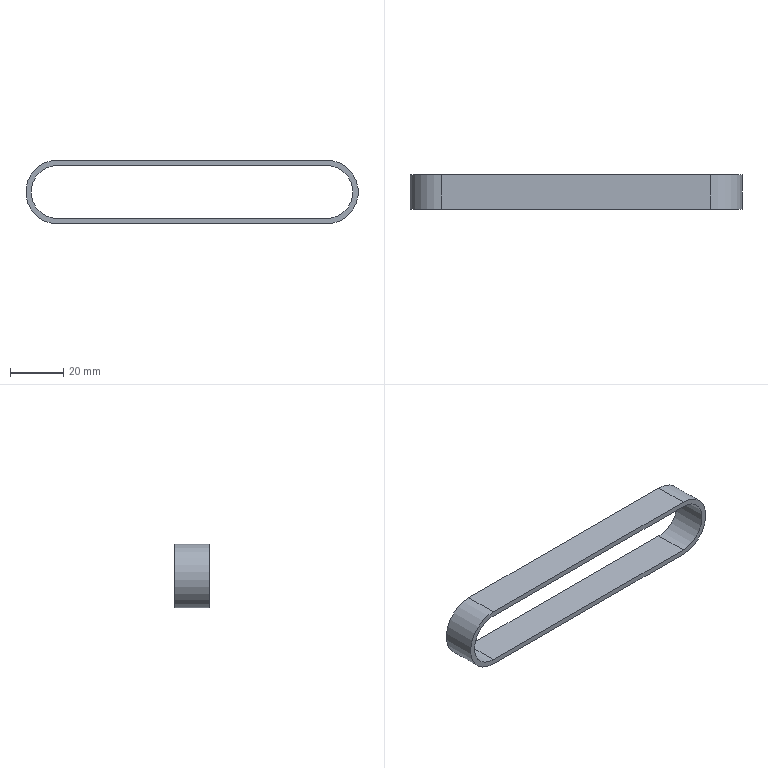Part | SolidWorks | features BaseBody 1 | 1 solid | 10 faces | box 125 x 13 x 24 mm | volume 7049 mm3 | plane 6 | cylinder 4 | commonest cylinder face diameters 20 x2 24 x2
STEP:
#1=CARTESIAN_POINT('',(-43.753,647.757,-287.268));
#2=VERTEX_POINT('',#1);
#3=CARTESIAN_POINT('',(-43.753,634.757,-287.268));
#4=VERTEX_POINT('',#3);
#5=CARTESIAN_POINT('',(-43.753,647.757,-287.268));
#6=DIRECTION('',(0.,-1.,0.));
#7=VECTOR('',#6,1000.);
#8=LINE('',#5,#7);
#9=EDGE_CURVE('',#2,#4,#8,.T.);
#10=ORIENTED_EDGE('',*,*,#9,.T.);
#11=CARTESIAN_POINT('',(57.247,634.757,-287.268));
#12=VERTEX_POINT('',#11);
#13=CARTESIAN_POINT('',(57.247,634.757,-287.268));
#14=DIRECTION('',(1.,0.,0.));
#15=VECTOR('',#14,1000.);
#16=LINE('',#13,#15);
#17=EDGE_CURVE('',#4,#12,#16,.T.);
#18=ORIENTED_EDGE('',*,*,#17,.T.);
#19=CARTESIAN_POINT('',(57.247,647.757,-287.268));
#20=VERTEX_POINT('',#19);
#21=CARTESIAN_POINT('',(57.247,647.757,-287.268));
#22=DIRECTION('',(0.,1.,0.));
#23=VECTOR('',#22,1000.);
#24=LINE('',#21,#23);
#25=EDGE_CURVE('',#12,#20,#24,.T.);
#26=ORIENTED_EDGE('',*,*,#25,.T.);
#27=CARTESIAN_POINT('',(57.247,647.757,-287.268));
#28=DIRECTION('',(-1.,0.,0.));
#29=VECTOR('',#28,1000.);
#30=LINE('',#27,#29);
#31=EDGE_CURVE('',#20,#2,#30,.T.);
#32=ORIENTED_EDGE('',*,*,#31,.T.);
#33=EDGE_LOOP('',(#10,#18,#26,#32));
#34=FACE_OUTER_BOUND('',#33,.T.);
#35=CARTESIAN_POINT('',(57.247,647.757,-287.268));
#36=DIRECTION('',(0.,0.,1.));
#37=DIRECTION('',(1.,0.,0.));
#38=AXIS2_PLACEMENT_3D('',#35,#36,#37);
#39=PLANE('',#38);
#40=ADVANCED_FACE('',(#34),#39,.T.);
#41=CARTESIAN_POINT('',(-43.753,634.757,-309.268));
#42=VERTEX_POINT('',#41);
#43=CARTESIAN_POINT('',(57.247,634.757,-309.268));
#44=VERTEX_POINT('',#43);
#45=CARTESIAN_POINT('',(57.247,634.757,-309.268));
#46=DIRECTION('',(1.,0.,0.));
#47=VECTOR('',#46,1000.);
#48=LINE('',#45,#47);
#49=EDGE_CURVE('',#42,#44,#48,.T.);
#50=ORIENTED_EDGE('',*,*,#49,.F.);
#51=CARTESIAN_POINT('',(-43.753,634.757,-289.268));
#52=VERTEX_POINT('',#51);
#53=CARTESIAN_POINT('',(-43.753,634.757,-299.268));
#54=DIRECTION('',(0.,-1.,0.));
#55=DIRECTION('',(0.,0.,-1.));
#56=AXIS2_PLACEMENT_3D('',#53,#54,#55);
#57=CIRCLE('',#56,10.);
#58=EDGE_CURVE('',#52,#42,#57,.T.);
#59=ORIENTED_EDGE('',*,*,#58,.F.);
#60=CARTESIAN_POINT('',(57.247,634.757,-289.268));
#61=VERTEX_POINT('',#60);
#62=CARTESIAN_POINT('',(57.247,634.757,-289.268));
#63=DIRECTION('',(-1.,0.,0.));
#64=VECTOR('',#63,1000.);
#65=LINE('',#62,#64);
#66=EDGE_CURVE('',#61,#52,#65,.T.);
#67=ORIENTED_EDGE('',*,*,#66,.F.);
#68=CARTESIAN_POINT('',(57.247,634.757,-299.268));
#69=DIRECTION('',(0.,-1.,0.));
#70=DIRECTION('',(0.,0.,-1.));
#71=AXIS2_PLACEMENT_3D('',#68,#69,#70);
#72=CIRCLE('',#71,10.);
#73=EDGE_CURVE('',#44,#61,#72,.T.);
#74=ORIENTED_EDGE('',*,*,#73,.F.);
#75=EDGE_LOOP('',(#50,#59,#67,#74));
#76=FACE_BOUND('',#75,.T.);
#77=CARTESIAN_POINT('',(57.247,634.757,-311.268));
#78=VERTEX_POINT('',#77);
#79=CARTESIAN_POINT('',(-43.753,634.757,-311.268));
#80=VERTEX_POINT('',#79);
#81=CARTESIAN_POINT('',(57.247,634.757,-311.268));
#82=DIRECTION('',(-1.,0.,0.));
#83=VECTOR('',#82,1000.);
#84=LINE('',#81,#83);
#85=EDGE_CURVE('',#78,#80,#84,.T.);
#86=ORIENTED_EDGE('',*,*,#85,.F.);
#87=CARTESIAN_POINT('',(57.247,634.757,-299.268));
#88=DIRECTION('',(0.,1.,0.));
#89=DIRECTION('',(0.,0.,-1.));
#90=AXIS2_PLACEMENT_3D('',#87,#88,#89);
#91=CIRCLE('',#90,12.);
#92=EDGE_CURVE('',#12,#78,#91,.T.);
#93=ORIENTED_EDGE('',*,*,#92,.F.);
#94=ORIENTED_EDGE('',*,*,#17,.F.);
#95=CARTESIAN_POINT('',(-43.753,634.757,-299.268));
#96=DIRECTION('',(0.,1.,0.));
#97=DIRECTION('',(0.,0.,-1.));
#98=AXIS2_PLACEMENT_3D('',#95,#96,#97);
#99=CIRCLE('',#98,12.);
#100=EDGE_CURVE('',#80,#4,#99,.T.);
#101=ORIENTED_EDGE('',*,*,#100,.F.);
#102=EDGE_LOOP('',(#86,#93,#94,#101));
#103=FACE_OUTER_BOUND('',#102,.T.);
#104=CARTESIAN_POINT('',(57.247,634.757,-289.268));
#105=DIRECTION('',(0.,1.,0.));
#106=DIRECTION('',(0.,0.,1.));
#107=AXIS2_PLACEMENT_3D('',#104,#105,#106);
#108=PLANE('',#107);
#109=ADVANCED_FACE('',(#76,#103),#108,.F.);
#110=CARTESIAN_POINT('',(-43.753,647.757,-311.268));
#111=VERTEX_POINT('',#110);
#112=CARTESIAN_POINT('',(-43.753,647.757,-311.268));
#113=DIRECTION('',(0.,-1.,0.));
#114=VECTOR('',#113,1000.);
#115=LINE('',#112,#114);
#116=EDGE_CURVE('',#111,#80,#115,.T.);
#117=ORIENTED_EDGE('',*,*,#116,.T.);
#118=ORIENTED_EDGE('',*,*,#100,.T.);
#119=ORIENTED_EDGE('',*,*,#9,.F.);
#120=CARTESIAN_POINT('',(-43.753,647.757,-299.268));
#121=DIRECTION('',(0.,-1.,0.));
#122=DIRECTION('',(0.,0.,-1.));
#123=AXIS2_PLACEMENT_3D('',#120,#121,#122);
#124=CIRCLE('',#123,12.);
#125=EDGE_CURVE('',#2,#111,#124,.T.);
#126=ORIENTED_EDGE('',*,*,#125,.T.);
#127=EDGE_LOOP('',(#117,#118,#119,#126));
#128=FACE_OUTER_BOUND('',#127,.T.);
#129=CARTESIAN_POINT('',(-43.753,647.757,-299.268));
#130=DIRECTION('',(0.,-1.,0.));
#131=DIRECTION('',(0.,0.,-1.));
#132=AXIS2_PLACEMENT_3D('',#129,#130,#131);
#133=CYLINDRICAL_SURFACE('',#132,12.);
#134=ADVANCED_FACE('',(#128),#133,.T.);
#135=CARTESIAN_POINT('',(-43.753,647.757,-289.268));
#136=VERTEX_POINT('',#135);
#137=CARTESIAN_POINT('',(-43.753,647.757,-309.268));
#138=VERTEX_POINT('',#137);
#139=CARTESIAN_POINT('',(-43.753,647.757,-299.268));
#140=DIRECTION('',(0.,-1.,0.));
#141=DIRECTION('',(0.,0.,-1.));
#142=AXIS2_PLACEMENT_3D('',#139,#140,#141);
#143=CIRCLE('',#142,10.);
#144=EDGE_CURVE('',#136,#138,#143,.T.);
#145=ORIENTED_EDGE('',*,*,#144,.T.);
#146=CARTESIAN_POINT('',(57.247,647.757,-309.268));
#147=VERTEX_POINT('',#146);
#148=CARTESIAN_POINT('',(-43.753,647.757,-309.268));
#149=DIRECTION('',(1.,0.,0.));
#150=VECTOR('',#149,1000.);
#151=LINE('',#148,#150);
#152=EDGE_CURVE('',#138,#147,#151,.T.);
#153=ORIENTED_EDGE('',*,*,#152,.T.);
#154=CARTESIAN_POINT('',(57.247,647.757,-289.268));
#155=VERTEX_POINT('',#154);
#156=CARTESIAN_POINT('',(57.247,647.757,-299.268));
#157=DIRECTION('',(0.,-1.,0.));
#158=DIRECTION('',(0.,0.,-1.));
#159=AXIS2_PLACEMENT_3D('',#156,#157,#158);
#160=CIRCLE('',#159,10.);
#161=EDGE_CURVE('',#147,#155,#160,.T.);
#162=ORIENTED_EDGE('',*,*,#161,.T.);
#163=CARTESIAN_POINT('',(-43.753,647.757,-289.268));
#164=DIRECTION('',(-1.,0.,0.));
#165=VECTOR('',#164,1000.);
#166=LINE('',#163,#165);
#167=EDGE_CURVE('',#155,#136,#166,.T.);
#168=ORIENTED_EDGE('',*,*,#167,.T.);
#169=EDGE_LOOP('',(#145,#153,#162,#168));
#170=FACE_BOUND('',#169,.T.);
#171=CARTESIAN_POINT('',(57.247,647.757,-311.268));
#172=VERTEX_POINT('',#171);
#173=CARTESIAN_POINT('',(57.247,647.757,-299.268));
#174=DIRECTION('',(0.,1.,0.));
#175=DIRECTION('',(0.,0.,-1.));
#176=AXIS2_PLACEMENT_3D('',#173,#174,#175);
#177=CIRCLE('',#176,12.);
#178=EDGE_CURVE('',#20,#172,#177,.T.);
#179=ORIENTED_EDGE('',*,*,#178,.T.);
#180=CARTESIAN_POINT('',(-43.753,647.757,-311.268));
#181=DIRECTION('',(-1.,0.,0.));
#182=VECTOR('',#181,1000.);
#183=LINE('',#180,#182);
#184=EDGE_CURVE('',#172,#111,#183,.T.);
#185=ORIENTED_EDGE('',*,*,#184,.T.);
#186=ORIENTED_EDGE('',*,*,#125,.F.);
#187=ORIENTED_EDGE('',*,*,#31,.F.);
#188=EDGE_LOOP('',(#179,#185,#186,#187));
#189=FACE_OUTER_BOUND('',#188,.T.);
#190=CARTESIAN_POINT('',(-43.753,647.757,-309.268));
#191=DIRECTION('',(0.,1.,0.));
#192=DIRECTION('',(0.,0.,1.));
#193=AXIS2_PLACEMENT_3D('',#190,#191,#192);
#194=PLANE('',#193);
#195=ADVANCED_FACE('',(#170,#189),#194,.T.);
#196=ORIENTED_EDGE('',*,*,#25,.F.);
#197=ORIENTED_EDGE('',*,*,#92,.T.);
#198=CARTESIAN_POINT('',(57.247,647.757,-311.268));
#199=DIRECTION('',(0.,1.,0.));
#200=VECTOR('',#199,1000.);
#201=LINE('',#198,#200);
#202=EDGE_CURVE('',#78,#172,#201,.T.);
#203=ORIENTED_EDGE('',*,*,#202,.T.);
#204=ORIENTED_EDGE('',*,*,#178,.F.);
#205=EDGE_LOOP('',(#196,#197,#203,#204));
#206=FACE_OUTER_BOUND('',#205,.T.);
#207=CARTESIAN_POINT('',(57.247,647.757,-299.268));
#208=DIRECTION('',(0.,-1.,0.));
#209=DIRECTION('',(0.,0.,-1.));
#210=AXIS2_PLACEMENT_3D('',#207,#208,#209);
#211=CYLINDRICAL_SURFACE('',#210,12.);
#212=ADVANCED_FACE('',(#206),#211,.T.);
#213=ORIENTED_EDGE('',*,*,#161,.F.);
#214=CARTESIAN_POINT('',(57.247,647.757,-309.268));
#215=DIRECTION('',(0.,1.,0.));
#216=VECTOR('',#215,1000.);
#217=LINE('',#214,#216);
#218=EDGE_CURVE('',#44,#147,#217,.T.);
#219=ORIENTED_EDGE('',*,*,#218,.F.);
#220=ORIENTED_EDGE('',*,*,#73,.T.);
#221=CARTESIAN_POINT('',(57.247,647.757,-289.268));
#222=DIRECTION('',(0.,-1.,0.));
#223=VECTOR('',#222,1000.);
#224=LINE('',#221,#223);
#225=EDGE_CURVE('',#155,#61,#224,.T.);
#226=ORIENTED_EDGE('',*,*,#225,.F.);
#227=EDGE_LOOP('',(#213,#219,#220,#226));
#228=FACE_OUTER_BOUND('',#227,.T.);
#229=CARTESIAN_POINT('',(57.247,647.757,-299.268));
#230=DIRECTION('',(0.,-1.,0.));
#231=DIRECTION('',(0.,0.,-1.));
#232=AXIS2_PLACEMENT_3D('',#229,#230,#231);
#233=CYLINDRICAL_SURFACE('',#232,10.);
#234=ADVANCED_FACE('',(#228),#233,.F.);
#235=ORIENTED_EDGE('',*,*,#152,.F.);
#236=CARTESIAN_POINT('',(-43.753,647.757,-309.268));
#237=DIRECTION('',(0.,1.,0.));
#238=VECTOR('',#237,1000.);
#239=LINE('',#236,#238);
#240=EDGE_CURVE('',#42,#138,#239,.T.);
#241=ORIENTED_EDGE('',*,*,#240,.F.);
#242=ORIENTED_EDGE('',*,*,#49,.T.);
#243=ORIENTED_EDGE('',*,*,#218,.T.);
#244=EDGE_LOOP('',(#235,#241,#242,#243));
#245=FACE_OUTER_BOUND('',#244,.T.);
#246=CARTESIAN_POINT('',(-43.753,647.757,-309.268));
#247=DIRECTION('',(0.,0.,-1.));
#248=DIRECTION('',(-1.,0.,0.));
#249=AXIS2_PLACEMENT_3D('',#246,#247,#248);
#250=PLANE('',#249);
#251=ADVANCED_FACE('',(#245),#250,.F.);
#252=ORIENTED_EDGE('',*,*,#144,.F.);
#253=CARTESIAN_POINT('',(-43.753,647.757,-289.268));
#254=DIRECTION('',(0.,1.,0.));
#255=VECTOR('',#254,1000.);
#256=LINE('',#253,#255);
#257=EDGE_CURVE('',#52,#136,#256,.T.);
#258=ORIENTED_EDGE('',*,*,#257,.F.);
#259=ORIENTED_EDGE('',*,*,#58,.T.);
#260=ORIENTED_EDGE('',*,*,#240,.T.);
#261=EDGE_LOOP('',(#252,#258,#259,#260));
#262=FACE_OUTER_BOUND('',#261,.T.);
#263=CARTESIAN_POINT('',(-43.753,647.757,-299.268));
#264=DIRECTION('',(0.,-1.,0.));
#265=DIRECTION('',(0.,0.,-1.));
#266=AXIS2_PLACEMENT_3D('',#263,#264,#265);
#267=CYLINDRICAL_SURFACE('',#266,10.);
#268=ADVANCED_FACE('',(#262),#267,.F.);
#269=ORIENTED_EDGE('',*,*,#167,.F.);
#270=ORIENTED_EDGE('',*,*,#225,.T.);
#271=ORIENTED_EDGE('',*,*,#66,.T.);
#272=ORIENTED_EDGE('',*,*,#257,.T.);
#273=EDGE_LOOP('',(#269,#270,#271,#272));
#274=FACE_OUTER_BOUND('',#273,.T.);
#275=CARTESIAN_POINT('',(57.247,647.757,-289.268));
#276=DIRECTION('',(0.,0.,1.));
#277=DIRECTION('',(1.,0.,0.));
#278=AXIS2_PLACEMENT_3D('',#275,#276,#277);
#279=PLANE('',#278);
#280=ADVANCED_FACE('',(#274),#279,.F.);
#281=ORIENTED_EDGE('',*,*,#202,.F.);
#282=ORIENTED_EDGE('',*,*,#85,.T.);
#283=ORIENTED_EDGE('',*,*,#116,.F.);
#284=ORIENTED_EDGE('',*,*,#184,.F.);
#285=EDGE_LOOP('',(#281,#282,#283,#284));
#286=FACE_OUTER_BOUND('',#285,.T.);
#287=CARTESIAN_POINT('',(-43.753,647.757,-311.268));
#288=DIRECTION('',(0.,0.,-1.));
#289=DIRECTION('',(-1.,0.,0.));
#290=AXIS2_PLACEMENT_3D('',#287,#288,#289);
#291=PLANE('',#290);
#292=ADVANCED_FACE('',(#286),#291,.T.);
#293=CLOSED_SHELL('',(#40,#109,#134,#195,#212,#234,#251,#268,#280,#292));
#294=MANIFOLD_SOLID_BREP('',#293);
#295=CARTESIAN_POINT('',(0.,0.,0.));
#296=DIRECTION('',(0.,0.,1.));
#297=DIRECTION('',(1.,0.,0.));
#298=AXIS2_PLACEMENT_3D('',#295,#296,#297);
#299=(LENGTH_UNIT()NAMED_UNIT(*)SI_UNIT(.MILLI.,.METRE.));
#300=UNCERTAINTY_MEASURE_WITH_UNIT(LENGTH_MEASURE(0.00001),#299,'','');
#301=(NAMED_UNIT(*)PLANE_ANGLE_UNIT()SI_UNIT($,.RADIAN.));
#302=(NAMED_UNIT(*)SI_UNIT($,.STERADIAN.)SOLID_ANGLE_UNIT());
#303=(GEOMETRIC_REPRESENTATION_CONTEXT(3)GLOBAL_UNCERTAINTY_ASSIGNED_CONTEXT((#300))GLOBAL_UNIT_ASSIGNED_CONTEXT((#299,#301,#302))REPRESENTATION_CONTEXT('',''));
#304=ADVANCED_BREP_SHAPE_REPRESENTATION('',(#294,#298),#303);